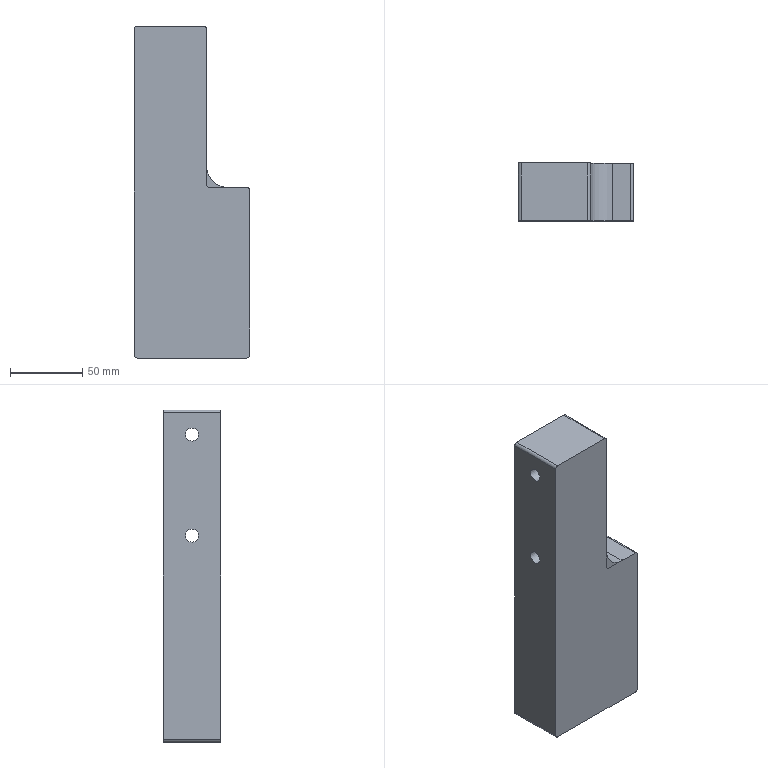NC program | NX | posted with a generic post | part box 80 x 40 x 230 mm
Lines 11596 to 12419 of 15398:
(PLANAR_MILL_COPY_COPY_1_COPY_1_COPY , TOOL : D10.)
N23148 T01 M6
N23150 G53
N23152 G17 G0 G90 X0.274 Y53.985 B0. C0. S3500 M3
N23154 G43 Z50. H1
N23156 Z4.6 B-180.
N23158 G41 G94 G1 X0.1 Y53. F1500. D1
N23160 Y38.
N23162 Y25.1
N23164 G3 X18.1 Y7.1 R18.
N23166 G1 X113.
N23168 X128.
N23170 G40
N23172 X128.985 Y7.274
N23174 G0 Z11.
N23176 X0.274 Y53.985
N23178 Z4.2
N23180 G41 G1 X0.1 Y53.
N23182 Y38.
N23184 Y25.1
N23186 G3 X18.1 Y7.1 R18.
N23188 G1 X113.
N23190 X128.
N23192 G40
N23194 X128.985 Y7.274
N23196 G0 Z10.6
N23198 X0.274 Y53.985
N23200 Z3.8
N23202 G41 G1 X0.1 Y53.
N23204 Y38.
N23206 Y25.1
N23208 G3 X18.1 Y7.1 R18.
N23210 G1 X113.
N23212 X128.
N23214 G40
N23216 X128.985 Y7.274
N23218 G0 Z10.2
N23220 X0.274 Y53.985
N23222 Z3.4
N23224 G41 G1 X0.1 Y53.
N23226 Y38.
N23228 Y25.1
N23230 G3 X18.1 Y7.1 R18.
N23232 G1 X113.
N23234 X128.
N23236 G40
N23238 X128.985 Y7.274
N23240 G0 Z9.8
N23242 X0.274 Y53.985
N23244 Z3.
N23246 G41 G1 X0.1 Y53.
N23248 Y38.
N23250 Y25.1
N23252 G3 X18.1 Y7.1 R18.
N23254 G1 X113.
N23256 X128.
N23258 G40
N23260 X128.985 Y7.274
N23262 G0 Z9.4
N23264 X0.274 Y53.985
N23266 Z2.6
N23268 G41 G1 X0.1 Y53.
N23270 Y38.
N23272 Y25.1
N23274 G3 X18.1 Y7.1 R18.
N23276 G1 X113.
N23278 X128.
N23280 G40
N23282 X128.985 Y7.274
N23284 G0 Z9.
N23286 X0.274 Y53.985
N23288 Z2.2
N23290 G41 G1 X0.1 Y53.
N23292 Y38.
N23294 Y25.1
N23296 G3 X18.1 Y7.1 R18.
N23298 G1 X113.
N23300 X128.
N23302 G40
N23304 X128.985 Y7.274
N23306 G0 Z8.6
N23308 X0.274 Y53.985
N23310 Z1.8
N23312 G41 G1 X0.1 Y53.
N23314 Y38.
N23316 Y25.1
N23318 G3 X18.1 Y7.1 R18.
N23320 G1 X113.
N23322 X128.
N23324 G40
N23326 X128.985 Y7.274
N23328 G0 Z8.2
N23330 X0.274 Y53.985
N23332 Z1.4
N23334 G41 G1 X0.1 Y53.
N23336 Y38.
N23338 Y25.1
N23340 G3 X18.1 Y7.1 R18.
N23342 G1 X113.
N23344 X128.
N23346 G40
N23348 X128.985 Y7.274
N23350 G0 Z7.8
N23352 X0.274 Y53.985
N23354 Z1.
N23356 G41 G1 X0.1 Y53.
N23358 Y38.
N23360 Y25.1
N23362 G3 X18.1 Y7.1 R18.
N23364 G1 X113.
N23366 X128.
N23368 G40
N23370 X128.985 Y7.274
N23372 G0 Z7.4
N23374 X0.274 Y53.985
N23376 Z0.6
N23378 G41 G1 X0.1 Y53.
N23380 Y38.
N23382 Y25.1
N23384 G3 X18.1 Y7.1 R18.
N23386 G1 X113.
N23388 X128.
N23390 G40
N23392 X128.985 Y7.274
N23394 G0 Z7.
N23396 X0.274 Y53.985
N23398 Z0.2
N23400 G41 G1 X0.1 Y53.
N23402 Y38.
N23404 Y25.1
N23406 G3 X18.1 Y7.1 R18.
N23408 G1 X113.
N23410 X128.
N23412 G40
N23414 X128.985 Y7.274
N23416 G0 Z6.6
N23418 X0.274 Y53.985
N23420 Z0.05
N23422 G41 G1 X0.1 Y53.
N23424 Y38.
N23426 Y25.1
N23428 G3 X18.1 Y7.1 R18.
N23430 G1 X113.
N23432 X128.
N23434 G40
N23436 X128.985 Y7.274
N23438 G0 Z50.
(ADAPTIVE_MILLING_COPY , TOOL : D10.)
N23440 X131.093 Y-42.154
N23442 Z3.05
N23444 G1 X130.949 Y-42.111 Z2.113 F3500.
N23446 X130.805 Y-42.068 Z1.742
N23448 X130.662 Y-42.025 Z1.47
N23450 X130.518 Y-41.982 Z1.25
N23452 X130.374 Y-41.939 Z1.066
N23454 X130.231 Y-41.896 Z0.908
N23456 X130.087 Y-41.853 Z0.77
N23458 X129.943 Y-41.81 Z0.65
N23460 X129.799 Y-41.767 Z0.545
N23462 X129.656 Y-41.724 Z0.452
N23464 X129.512 Y-41.681 Z0.371
N23466 X129.368 Y-41.638 Z0.3
N23468 X129.225 Y-41.595 Z0.24
N23470 X129.081 Y-41.552 Z0.188
N23472 X128.937 Y-41.509 Z0.145
N23474 X128.794 Y-41.466 Z0.111
N23476 X128.65 Y-41.423 Z0.084
N23478 X128.506 Y-41.38 Z0.065
N23480 X128.362 Y-41.337 Z0.054
N23482 X128.219 Y-41.294 Z0.05
N23484 X126.737 Y-40.85
N23486 G3 X125.467 Y-41.5 R1.047
N23488 G2 X123.725 Y-44.52 R40.399
N23490 X113.561 Y-50.458 R13.178
N23492 X107.135 Y-50.645 R78.774
N23494 G1 X-112.146 Y-50.635
N23496 G2 X-119.446 Y-48.637 R14.273
N23498 X-125.425 Y-38.867 R12.704
N23500 X-125.642 Y-32.835 R60.228
N23502 G1 X-125.639 Y36.996
N23504 G2 X-123.804 Y44.164 R14.479
N23506 X-113.788 Y50.434 R12.722
N23508 X-107.1 Y50.645 R72.946
N23510 G1 X0.181 Y50.637
N23512 G2 X7.374 Y48.74 R14.374
N23514 X13.522 Y38.896 R12.689
N23516 X13.745 Y32.297 R68.499
N23518 G3 X13.781 Y25.77 R248.361
N23520 X14.736 Y22.698 R5.595
N23522 X17.956 Y20.946 R4.399
N23524 X23.628 Y20.757 R59.107
N23526 G1 X111.896 Y20.742
N23528 G2 X118.927 Y19.038 R14.652
N23530 X125.426 Y8.959 R12.697
N23532 X125.642 Y2.928 R63.923
N23534 G1 X125.648 Y-36.497
N23536 G2 X123.98 Y-43.122 R12.586
N23538 X114.415 Y-49.838 R13.005
N23540 X108.618 Y-50.263 R39.297
N23542 X101.006 Y-50.3 R399.557
N23544 G1 X-111.196 Y-50.285
N23546 G2 X-117.348 Y-49.114 R16.471
N23548 X-124.778 Y-39.707 R12.409
N23550 X-125.256 Y-33.958 R35.302
N23552 X-125.299 Y-26.302 R339.034
N23554 G1 X-125.286 Y36.151
N23556 G2 X-124.163 Y42.228 R16.617
N23558 X-114.731 Y49.773 R12.402
N23560 X-108.721 Y50.261 R36.157
N23562 X-101.327 Y50.3 R362.187
N23564 G1 X-0.761 Y50.287
N23566 G2 X5.395 Y49.136 R16.577
N23568 X12.864 Y39.782 R12.391
N23570 X13.358 Y33.86 R35.329
N23572 G3 X13.435 Y26.558 R609.202
N23574 X14.161 Y23.314 R7.837
N23576 X17.726 Y20.79 R4.746
N23578 X22.393 Y20.443 R30.407
N23580 G1 X28.727 Y20.4
N23582 X111.114 Y20.387
N23584 G2 X117.231 Y19.262 R16.664
N23586 X124.759 Y9.903 R12.385
N23588 X125.257 Y4.025 R34.9
N23590 X125.3 Y-4.024 R361.131
N23592 G1 X125.289 Y-36.046
N23594 G2 X120.717 Y-46.35 R13.767
N23596 X114.248 Y-49.357 R13.562
N23598 X107.717 Y-49.904 R39.151
N23600 X100.017 Y-49.949 R337.307
N23602 G1 X-110.077 Y-49.939
N23604 G2 X-115.86 Y-49.124 R19.472
N23606 X-124.107 Y-40.288 R12.233
N23608 X-124.849 Y-34.484 R27.643
N23610 X-124.949 Y-24.816 R232.25
N23612 G1 X-124.936 Y35.259
N23614 G2 X-124.01 Y41.198 R18.667
N23616 X-115.359 Y49.088 R12.207
N23618 X-109.252 Y49.858 R28.129
N23620 X-99.803 Y49.949 R240.874
N23622 G1 X-1.753 Y49.938
N23624 G2 X4.068 Y49.089 R19.168
N23626 X12.203 Y40.301 R12.225
N23628 X12.954 Y34.366 R27.929
N23630 X13.08 Y27.438 R538.601
N23632 G3 X13.725 Y23.8 R10.769
N23634 X17.429 Y20.658 R5.131
N23636 X21.878 Y20.146 R22.319
N23638 X32.489 Y20.05 R321.794
N23640 G1 X110.277 Y20.036
N23642 G2 X116.173 Y19.119 R18.671
N23644 X124.094 Y10.433 R12.215
N23646 X124.845 Y4.674 R27.274
N23648 X124.949 Y-3.988 R198.27
N23650 G1 X124.938 Y-35.083
N23652 G2 X123.293 Y-42.177 R15.764
N23654 X115.323 Y-48.572 R12.671
N23656 X109.058 Y-49.472 R27.358
N23658 X98.122 Y-49.599 R259.091
N23660 G1 X-109.445 Y-49.585
N23662 G2 X-115.152 Y-48.832 R20.966
N23664 X-123.507 Y-40.447 R12.18
N23666 X-124.445 Y-34.498 R25.294
N23668 X-124.599 Y-23.825 R209.43
N23670 G1 X-124.588 Y34.27
N23672 G2 X-123.869 Y40.026 R21.602
N23674 X-115.528 Y48.482 R12.165
N23676 X-109.495 Y49.445 R25.079
N23678 X-100.397 Y49.598 R165.674
N23680 G1 X-2.642 Y49.588
N23682 G2 X3.03 Y48.897 R21.793
N23684 X11.599 Y40.475 R12.182
N23686 X12.556 Y34.309 R25.658
N23688 X12.739 Y27.832 R490.44
N23690 G3 X13.429 Y23.969 R12.316
N23692 X17.415 Y20.456 R5.669
N23694 X22.181 Y19.827 R22.029
N23696 X31.484 Y19.7 R199.522
N23698 G1 X109.321 Y19.688
N23700 G2 X115.117 Y18.942 R21.289
N23702 X123.491 Y10.599 R12.168
N23704 X124.45 Y4.521 R25.332
N23706 X124.598 Y-4.796 R186.673
N23708 G1 X124.586 Y-34.202
N23710 G2 X123.484 Y-40.504 R17.988
N23712 X115.532 Y-47.956 R12.572
N23714 X109.214 Y-49.061 R24.942
N23716 X100.293 Y-49.247 R142.121
N23718 G1 X-108.576 Y-49.236
N23720 G2 X-114.425 Y-48.542 R23.063
N23722 X-122.924 Y-40.51 R12.175
N23724 X-124.044 Y-34.373 R23.938
N23726 X-124.247 Y-25.321 R141.619
N23728 G1 X-124.235 Y33.616
N23730 G2 X-123.555 Y39.379 R23.087
N23732 X-115.513 Y47.923 R12.178
N23734 X-109.377 Y49.044 R23.937
N23736 X-99.45 Y49.248 R154.683
N23738 G1 X-3.281 Y49.235
N23740 G2 X2.524 Y48.542 R22.961
N23742 X11.021 Y40.522 R12.172
N23744 X12.156 Y34.211 R24.261
N23746 X12.401 Y28.105 R502.905
N23748 G3 X13.157 Y24.057 R13.32
N23750 X17.299 Y20.275 R6.168
N23752 X22.116 Y19.527 R20.663
N23754 X31.879 Y19.35 R179.371
N23756 G1 X108.664 Y19.335
N23758 G2 X114.51 Y18.618 R22.679
N23760 X122.918 Y10.626 R12.171
N23762 X124.046 Y4.445 R23.951
N23764 X124.246 Y-4.432 R136.352
N23766 G1 X124.234 Y-33.42
N23768 G2 X123.335 Y-39.454 R20.013
N23770 X115.476 Y-47.417 R12.566
N23772 X109.009 Y-48.667 R24.183
N23774 X100.045 Y-48.895 R130.758
N23776 G1 X-107.827 Y-48.886
N23778 G2 X-113.685 Y-48.252 R25.051
N23780 X-122.425 Y-40.317 R12.256
N23782 X-123.659 Y-34.024 R23.668
N23784 X-123.893 Y-25.411 R121.991
N23786 G1 X-123.885 Y32.827
N23788 G2 X-123.284 Y38.557 R25.399
N23790 X-115.388 Y47.398 R12.244
N23792 X-109.056 Y48.656 R23.442
N23794 X-99.962 Y48.895 R126.676
N23796 G1 X-4.042 Y48.885
N23798 G2 X1.815 Y48.244 R24.896
N23800 X10.499 Y40.388 R12.237
N23802 X11.749 Y34.143 R23.32
N23804 X12.06 Y28.335 R420.196
N23806 G3 X12.949 Y23.966 R14.108
N23808 X17.196 Y20.085 R6.681
N23810 X21.97 Y19.237 R19.678
N23812 X31.014 Y19.005 R133.329
N23814 G1 X107.914 Y18.985
N23816 G2 X113.685 Y18.352 R24.815
N23818 X122.388 Y10.516 R12.231
N23820 X123.643 Y4.317 R23.118
N23822 X123.894 Y-4.778 R120.904
N23824 G1 X123.889 Y-32.259
N23826 G2 X123.234 Y-38.113 R23.956
N23828 X115.235 Y-46.945 R12.637
N23830 X108.914 Y-48.262 R23.609
N23832 X100.127 Y-48.541 R110.359
N23834 G1 X-107.035 Y-48.536
N23836 G2 X-112.86 Y-47.977 R27.616
N23838 X-121.933 Y-40.111 R12.352
N23840 X-123.271 Y-33.707 R23.354
N23842 X-123.542 Y-24.657 R115.958
N23844 G1 X-123.533 Y32.224
N23846 G2 X-122.913 Y38.129 R26.218
N23848 X-115.244 Y46.88 R12.306
N23850 X-108.978 Y48.246 R22.651
N23852 X-100.104 Y48.541 R105.687
N23854 G1 X-4.679 Y48.533
N23856 G2 X1.14 Y47.934 R26.427
N23858 X10.024 Y40.132 R12.333
N23860 X11.37 Y33.729 R23.327
N23862 G3 X11.759 Y28.099 R694.113
N23864 X12.8 Y23.736 R13.63
N23866 X17.17 Y19.863 R7.234
N23868 X22.057 Y18.932 R19.665
N23870 X31.672 Y18.655 R125.783
N23872 G1 X107.219 Y18.634
N23874 G2 X112.996 Y18.045 R26.596
N23876 X121.936 Y10.202 R12.346
N23878 X123.276 Y3.754 R23.451
N23880 X123.542 Y-5.077 R114.881
N23882 G1 X123.536 Y-31.67
N23884 G2 X122.893 Y-37.571 R25.133
N23886 X115.093 Y-46.434 R12.673
N23888 X108.492 Y-47.887 R23.413
N23890 X99.137 Y-48.191 R111.429
N23892 G1 X-106.47 Y-48.184
N23894 G2 X-112.382 Y-47.618 R28.359
N23896 X-121.489 Y-39.788 R12.455
N23898 X-122.884 Y-33.396 R23.229
N23900 X-123.188 Y-24.698 R103.453
N23902 G1 X-123.187 Y31.252
N23904 G2 X-122.675 Y37.126 R30.064
N23906 X-118.101 Y44.631 R12.469
N23908 X-111.849 Y47.368 R15.515
N23910 X-104.896 Y48.099 R39.966
N23912 X-93.872 Y48.198 R302.972
N23914 G1 X-5.442 Y48.184
N23916 G2 X0.513 Y47.612 R28.32
N23918 X9.559 Y39.861 R12.438
N23920 X10.981 Y33.474 R23.211
N23922 G3 X11.449 Y28.016 R259.571
N23924 X12.625 Y23.571 R13.849
N23926 X17.138 Y19.637 R7.798
N23928 X22.297 Y18.612 R20.186
N23930 X31.853 Y18.308 R118.944
N23932 G1 X106.471 Y18.285
N23934 G2 X112.34 Y17.729 R28.522
N23936 X121.449 Y9.986 R12.437
N23938 X122.874 Y3.602 R22.893
N23940 X123.187 Y-5.096 R100.525
N23942 G1 X123.186 Y-30.915
N23944 G2 X122.612 Y-36.781 R27.524
N23946 X114.658 Y-46.044 R12.797
N23948 X108.235 Y-47.496 R23.405
N23950 X99.451 Y-47.834 R97.738
N23952 G1 X-105.611 Y-47.837
N23954 G2 X-111.532 Y-47.342 R31.559
N23956 X-118.935 Y-43.055 R12.628
N23958 X-121.91 Y-36.725 R15.278
N23960 X-122.722 Y-29.827 R37.431
N23962 X-122.848 Y-18.365 R308.19
N23964 G1 X-122.837 Y30.553
N23966 G2 X-122.345 Y36.518 R31.863
N23968 X-118.14 Y43.863 R12.641
N23970 X-111.964 Y46.852 R14.99
N23972 X-104.897 Y47.719 R36.261
N23974 X-93.392 Y47.848 R302.118
N23976 G1 X-6.324 Y47.837
N23978 G2 X-0.317 Y47.332 R31.493
N23980 X7.206 Y42.843 R12.587
N23982 X10.044 Y36.582 R15.539
N23984 X10.864 Y30.428 R45.557
N23986 G3 X11.667 Y25.393 R26.942
N23988 X14.38 Y20.967 R8.85
N23990 X18.692 Y18.909 R10.574
N23992 X24.902 Y18.12 R32.956
N23994 X35.772 Y17.949 R241.455
N23996 G1 X105.557 Y17.938
N23998 G2 X111.478 Y17.454 R32.015
N24000 X118.752 Y13.372 R12.681
N24002 X121.862 Y7.023 R15.005
N24004 X122.713 Y0.13 R36.108
N24006 X122.848 Y-11.418 R290.381
N24008 G1 X122.834 Y-30.358
N24010 G2 X122.263 Y-36.269 R28.459
N24012 X114.507 Y-45.541 R12.848
N24014 X107.89 Y-47.115 R23.083
N24016 X98.845 Y-47.483 R95.445
N24018 G1 X-104.983 Y-47.486
N24020 G2 X-110.992 Y-46.998 R32.777
N24022 X-118.475 Y-42.714 R12.751
N24024 X-121.52 Y-36.311 R15.438
N24026 X-122.37 Y-29.153 R38.015
N24028 X-122.497 Y-17.299 R320.42
N24030 G1 X-122.483 Y30.202
N24032 G2 X-121.972 Y36.12 R31.4
N24034 X-117.219 Y43.867 R12.659
N24036 X-110.841 Y46.627 R16.105
N24038 X-103.629 Y47.39 R41.585
N24040 X-92.298 Y47.497 R363.499
N24042 G1 X-6.886 Y47.486
N24044 G2 X-0.835 Y46.984 R32.349
N24046 X6.764 Y42.482 R12.708
N24048 X9.657 Y36.163 R15.742
N24050 X10.507 Y30.376 R47.607
N24052 G3 X11.417 Y25.294 R27.085
N24054 X14.586 Y20.533 R9.219
N24056 X19.239 Y18.511 R12.12
N24058 X25.918 Y17.749 R38.379
N24060 X37.564 Y17.598 R299.62
N24062 G1 X104.983 Y17.587
N24064 G2 X111.035 Y17.09 R32.587
N24066 X118.495 Y12.79 R12.732
N24068 X121.525 Y6.393 R15.451
N24070 X122.374 Y-0.853 R38.45
N24072 X122.497 Y-12.576 R326.291
N24074 G1 X122.485 Y-29.601
N24076 G2 X121.94 Y-35.647 R30.419
N24078 X114.121 Y-45.138 R12.958
N24080 X107.642 Y-46.724 R22.982
N24082 X98.818 Y-47.127 R87.849
N24084 G1 X91.643 Y-47.147
N24086 X-104.32 Y-47.136
N24088 G2 X-110.332 Y-46.678 R34.785
N24090 X-117.453 Y-42.998 R13.039
N24092 X-120.956 Y-36.582 R14.748
N24094 X-121.97 Y-29.491 R33.516
N24096 X-122.146 Y-19.125 R199.152
N24098 G1 X-122.136 Y29.312
N24100 G2 X-121.672 Y35.368 R34.557
N24102 X-117.804 Y42.637 R12.989
N24104 X-111.539 Y45.967 R14.883
N24106 X-104.492 Y46.97 R33.647
N24108 X-92.507 Y47.147 R242.977
N24110 G1 X-7.582 Y47.136
N24112 G2 X-1.527 Y46.671 R34.497
N24114 X5.739 Y42.802 R12.984
N24116 X9.068 Y36.551 R14.942
N24118 X10.02 Y31.346 R34.859
N24120 G3 X10.918 Y26.022 R39.676
N24122 X13.473 Y21.232 R10.716
N24124 X18.179 Y18.526 R10.794
N24126 X24.311 Y17.524 R28.636
N24128 X33.996 Y17.258 R149.398
N24130 G1 X104.333 Y17.237
N24132 G2 X110.431 Y16.76 R34.28
N24134 X117.763 Y12.767 R12.941
N24136 X121.022 Y6.436 R15.089
N24138 X121.977 Y-0.531 R34.606
N24140 X122.147 Y-11.51 R230.562
N24142 G1 X122.133 Y-29.045
N24144 G2 X121.629 Y-34.965 R32.049
N24146 X117.032 Y-42.77 R13.102
N24148 X110.613 Y-45.765 R16.137
N24150 X103.153 Y-46.661 R39.462
N24152 X90.555 Y-46.797 R331.416
N24154 G1 X-103.845 Y-46.784
N24156 G2 X-109.815 Y-46.331 R35.248
N24158 X-116.993 Y-42.66 R13.179
N24160 X-120.56 Y-36.203 R14.847
N24162 X-121.604 Y-29.119 R33.287
N24164 X-121.796 Y-17.965 R212.844
N24166 G1 X-121.782 Y29.02
N24168 G2 X-121.272 Y35.115 R32.987
N24170 X-116.589 Y42.928 R12.904
N24172 X-110.297 Y45.795 R16.136
N24174 X-102.878 Y46.666 R39.803
N24176 X-90.585 Y46.797 R333.437
N24178 G1 X-7.848 Y46.781
N24180 G2 X-1.797 Y46.275 R32.957
N24182 X7.865 Y38.461 R12.928
N24184 X9.442 Y32.601 R24.348
N24186 G3 X10.329 Y27.196 R97.299
N24188 X12.251 Y22.381 R13.7
N24190 X17.324 Y18.552 R10.31
N24192 X23.342 Y17.298 R24.031
N24194 X33.18 Y16.917 R113.098
N24196 G1 X41.543 Y16.898
N24198 X104.02 Y16.883
N24200 G2 X110.115 Y16.373 R33.025
N24202 X117.866 Y11.769 R12.914
N24204 X120.813 Y5.319 R16.137
N24206 X121.66 Y-1.884 R39.651
N24208 X121.797 Y-14.263 R321.24
N24210 G1 X121.78 Y-28.62
N24212 G2 X121.238 Y-34.667 R31.508
N24214 X113.331 Y-44.349 R13.167
N24216 X106.686 Y-45.998 R23.448
N24218 X97.687 Y-46.423 R88.148
N24220 G1 X90.031 Y-46.447
N24222 X-103.088 Y-46.436
N24224 G2 X-109.19 Y-46.003 R37.533
N24226 X-116.169 Y-42.677 R13.46
N24228 X-120.016 Y-36.324 R14.481
N24230 X-121.199 Y-29.352 R30.367
N24232 X-121.443 Y-19.076 R156.13
N24234 G1 X-121.436 Y28.093
N24236 G2 X-120.987 Y34.281 R36.989
N24238 X-117.515 Y41.34 R13.363
N24240 X-111.06 Y45.098 R14.709
N24242 X-103.945 Y46.226 R32.001
N24244 X-92.355 Y46.446 R199.332
N24246 G1 X-8.83 Y46.436
N24248 G2 X-2.641 Y45.991 R37.258
N24250 X4.452 Y42.503 R13.38
N24252 X8.145 Y36.271 R14.772
N24254 X9.251 Y31.323 R33.759
N24256 G3 X10.332 Y25.99 R44.29
N24258 X13.17 Y20.901 R11.86
N24260 X18.276 Y17.959 R12.01
N24262 X24.689 Y16.867 R29.997
N24264 X34.876 Y16.56 R145.374
N24266 G1 X103.105 Y16.537
N24268 G2 X109.207 Y16.101 R37.359
N24270 X116.253 Y12.698 R13.433
N24272 X120.07 Y6.249 R14.616
N24274 X121.223 Y-0.905 R31.645
N24276 X121.444 Y-11.007 R164.918
N24278 G1 X121.432 Y-27.864
N24280 G2 X120.924 Y-34.003 R33.789
N24282 X116.592 Y-41.688 R13.348
N24284 X110.13 Y-44.922 R15.947
N24286 X102.729 Y-45.921 R37.025
N24288 X92.056 Y-46.095 R206.92
N24290 G1 X-102.839 Y-46.082
N24292 G2 X-109.024 Y-45.592 R35.136
N24294 X-116.499 Y-41.545 R13.274
N24296 X-119.87 Y-35.113 R15.495
N24298 X-120.895 Y-28.025 R34.756
N24300 X-121.095 Y-17.003 R207.337
N24302 G1 X-121.081 Y27.839
N24304 G2 X-120.608 Y33.938 R35.587
N24306 X-116.781 Y41.279 R13.348
N24308 X-110.36 Y44.8 R15.206
N24310 X-103.236 Y45.882 R33.514
N24312 X-91.995 Y46.095 R200.244
N24314 G1 X-9.073 Y46.082
N24316 G2 X-2.888 Y45.594 R35.239
N24318 X4.595 Y41.551 R13.281
N24320 X7.893 Y35.48 R15.667
N24322 X9.168 Y29.659 R52.676
N24324 G3 X10.593 Y24.428 R25.72
N24326 X17.244 Y18.046 R11.311
N24328 X23.635 Y16.653 R25.135
N24330 X33.281 Y16.227 R105.798
N24332 G1 X44.475 Y16.198
N24334 X102.883 Y16.182
N24336 G2 X109.024 Y15.692 R34.901
N24338 X116.525 Y11.617 R13.269
N24340 X119.901 Y5.096 R15.588
N24342 X120.914 Y-2.215 R35.979
N24344 X121.095 Y-12.931 R203.177
N24346 G1 X121.079 Y-27.418
N24348 G2 X120.565 Y-33.557 R33.938
N24350 X116.21 Y-41.286 R13.444
N24352 X109.749 Y-44.537 R16.055
N24354 X102.438 Y-45.554 R36.605
N24356 X90.672 Y-45.746 R234.087
N24358 G1 X-101.877 Y-45.736
N24360 G2 X-108.069 Y-45.326 R40.381
N24362 X-114.981 Y-42.245 R13.906
N24364 X-119.181 Y-35.725 R14.462
N24366 X-120.456 Y-28.726 R29.583
N24368 X-120.741 Y-18.32 R145.964
N24370 G1 X-120.736 Y26.877
N24372 G2 X-120.325 Y33.069 R40.367
N24374 X-117.213 Y40.017 R13.891
N24376 X-110.8 Y44.155 R14.443
N24378 X-103.762 Y45.453 R29.337
N24380 X-93.312 Y45.741 R145.575
N24382 G1 X-9.918 Y45.735
N24384 G2 X-3.77 Y45.315 R39.508
N24386 X3.222 Y42.122 R13.83
N24388 X7.207 Y36.024 R14.711
N24390 X8.515 Y31.078 R33.756
N24392 G3 X9.843 Y25.621 R44.721
N24394 X13.202 Y20.224 R12.664
N24396 X18.772 Y17.257 R13.735
N24398 X25.872 Y16.142 R34.748
N24400 X36.794 Y15.856 R173.894
N24402 G1 X102.02 Y15.835
N24404 G2 X108.296 Y15.387 R38.29
N24406 X115.411 Y11.957 R13.656
N24408 X119.292 Y5.481 R14.831
N24410 X120.499 Y-1.753 R31.622
N24412 X120.744 Y-12.73 R175.896
N24414 X120.708 Y-27.864 R882.062
N24416 X120.009 Y-33.98 R27.735
N24418 X112.28 Y-43.126 R13.393
N24420 X105.398 Y-44.902 R23.651
N24422 X96.621 Y-45.362 R83.736
N24424 G1 X87.959 Y-45.396
N24426 X-101.485 Y-45.384
N24428 G2 X-107.633 Y-44.966 R40.002
N24430 X-114.587 Y-41.854 R13.99
N24432 X-118.81 Y-35.291 R14.585
N24434 X-120.098 Y-28.249 R29.851
N24436 X-120.39 Y-17.668 R147.013
N24438 G1 X-120.384 Y26.482
N24440 G2 X-119.944 Y32.759 R39.242
N24442 X-116.722 Y39.738 R13.878
N24444 X-110.199 Y43.84 R14.705
N24446 X-103.11 Y45.109 R30.352
N24448 X-92.747 Y45.39 R145.068
N24450 G1 X-10.648 Y45.386
N24452 G2 X-4.281 Y44.968 R41.261
N24454 X2.641 Y41.896 R14.034
N24456 X6.785 Y35.772 R14.793
N24458 X8.211 Y30.677 R35.375
N24460 G3 X9.671 Y25.247 R40.407
N24462 X13.729 Y19.464 R12.824
N24464 X19.459 Y16.786 R15.395
N24466 X26.874 Y15.753 R40.013
N24468 X39.19 Y15.499 R222.897
N24470 G1 X101.487 Y15.485
N24472 G2 X107.808 Y15.036 R38.976
N24474 X114.946 Y11.633 R13.798
N24476 X118.904 Y5.1 R14.902
N24478 X120.134 Y-2.13 R31.538
N24480 X120.392 Y-12.975 R167.463
N24482 X120.355 Y-27.426 R839.812
N24484 X119.651 Y-33.542 R27.828
N24486 X111.8 Y-42.782 R13.507
N24488 X104.916 Y-44.545 R23.989
N24490 X95.92 Y-45.013 R85.415
N24492 G1 X87.651 Y-45.046
N24494 X-101.18 Y-45.03
N24496 G2 X-107.369 Y-44.577 R38.242
N24498 X-114.575 Y-41.124 R13.891
N24500 X-118.496 Y-34.689 R14.98
N24502 X-119.768 Y-27.422 R31.212
N24504 X-120.041 Y-16.797 R156.215
N24506 G1 X-120.032 Y26.046
N24508 G2 X-119.585 Y32.323 R39.154
N24510 X-116.24 Y39.449 R13.944
N24512 X-109.709 Y43.49 R14.911
N24514 X-102.4 Y44.77 R31.257
N24516 X-91.555 Y45.042 R162.418
N24518 G1 X-11.005 Y45.034
N24520 G2 X-4.769 Y44.618 R41.024
N24522 X2.201 Y41.549 R14.179
N24524 X6.368 Y35.515 R14.963
N24526 X7.856 Y30.53 R35.164
N24528 G3 X9.452 Y25.015 R40.957
N24530 X14.059 Y18.914 R13.237
N24532 X20.091 Y16.342 R16.943
N24534 X28.134 Y15.355 R46.215
N24536 X40.107 Y15.148 R244.365
N24538 G1 X100.873 Y15.135
N24540 G2 X107.196 Y14.708 R40.72
N24542 X114.184 Y11.575 R14.091
N24544 X118.39 Y5.109 R14.646
N24546 X119.724 Y-1.923 R29.353
N24548 X120.037 Y-11.934 R130.889
N24550 X120.002 Y-26.99 R783.022
N24552 X119.292 Y-33.105 R27.948
N24554 X111.523 Y-42.348 R13.572
N24556 X104.784 Y-44.145 R23.551
N24558 X95.704 Y-44.657 R80.55
N24560 G1 X87.129 Y-44.695
N24562 X-100.434 Y-44.683
N24564 G2 X-106.713 Y-44.257 R40.981
N24566 X-113.652 Y-41.208 R14.266
N24568 X-118.021 Y-34.58 R14.704
N24570 X-119.382 Y-27.329 R29.96
N24572 X-119.688 Y-16.88 R141.175
N24574 G1 X-119.68 Y25.607
N24576 G2 X-119.228 Y31.884 R39.112
N24578 X-115.901 Y39.005 R14.058
N24580 X-109.43 Y43.072 R14.928
N24582 X-102.216 Y44.391 R30.521
N24584 X-92.029 Y44.688 R140.674
N24586 G1 X-11.436 Y44.682
N24588 G2 X-5.028 Y44.23 R39.929
N24590 X2.207 Y40.814 R14.077
N24592 X6.149 Y34.778 R15.722
N24594 X7.842 Y29.086 R53.078
N24596 G3 X9.754 Y23.656 R27.865
N24598 X17.268 Y16.922 R13.599
N24600 X24.044 Y15.368 R27.456
N24602 X34. Y14.844 R99.657
N24604 X48.41 Y14.797 R846.501
N24606 G1 X100.433 Y14.784
N24608 G2 X106.712 Y14.358 R40.968
N24610 X113.759 Y11.218 R14.236
N24612 X118.024 Y4.674 R14.756
N24614 X119.364 Y-2.357 R29.558
N24616 X119.685 Y-12.28 R126.711
N24618 X119.651 Y-26.508 R698.507
N24620 X118.936 Y-32.666 R28.195
N24622 X111.116 Y-41.974 R13.661
N24624 X104.249 Y-43.797 R23.829
N24626 X95.212 Y-44.306 R81.594
N24628 X85.981 Y-44.345 R596.713
N24630 G1 X-99.952 Y-44.332
N24632 G2 X-106.404 Y-43.878 R40.458
N24634 X-113.509 Y-40.61 R14.213
N24636 X-117.716 Y-33.971 R15.012
N24638 X-119.027 Y-26.844 R30.47
N24640 X-119.337 Y-16.482 R141.062
N24642 G1 X-119.335 Y24.602
N24644 G2 X-118.936 Y31.059 R44.421
N24646 X-116.114 Y37.904 R14.633
N24648 X-109.549 Y42.514 R14.518
N24650 X-102.583 Y43.961 R28.055
N24652 X-92.574 Y44.331 R117.347
N24654 G1 X-12.374 Y44.336
N24656 G2 X-5.917 Y43.948 R45.481
N24658 X0.958 Y41.154 R14.739
N24660 X5.496 Y35.119 R15.071
N24662 X7.164 Y30.182 R35.465
N24664 G3 X8.962 Y24.686 R42.982
N24666 X14.514 Y18.009 R14.27
N24668 X20.976 Y15.557 R19.616
N24670 X29.585 Y14.626 R54.287
N24672 X43.339 Y14.445 R355.381
N24674 G1 X99.824 Y14.434
N24676 G2 X106.234 Y14.008 R42.027
N24678 X113.254 Y10.93 R14.391
N24680 X117.605 Y4.395 R14.756
N24682 X118.994 Y-2.671 R29.185
N24684 X119.335 Y-13.075 R130.456
N24686 X119.292 Y-26.25 R543.955
N24688 X118.546 Y-32.36 R27.458
N24690 X110.703 Y-41.606 R13.746
N24692 X103.66 Y-43.457 R24.221
N24694 X94.579 Y-43.956 R83.971
N24696 X85.96 Y-43.995 R587.256
N24698 G1 X-99.546 Y-43.98
N24700 G2 X-105.911 Y-43.531 R40.524
N24702 X-113.036 Y-40.3 R14.375
N24704 X-117.299 Y-33.698 R15.019
N24706 X-118.662 Y-26.494 R30.306
N24708 X-118.987 Y-15.827 R140.665
N24710 G1 X-118.98 Y24.517
N24712 G2 X-118.521 Y30.969 R40.306
N24714 X-115.313 Y38.021 R14.332
N24716 X-108.773 Y42.273 R14.968
N24718 X-101.66 Y43.647 R29.805
N24720 X-91.343 Y43.985 R132.148
N24722 G1 X-12.368 Y43.98
N24724 G2 X-6.003 Y43.534 R40.749
N24726 X1.273 Y40.194 R14.437
N24728 X5.349 Y34.268 R16.104
N24730 X7.124 Y28.998 R51.89
N24732 G3 X9.292 Y23.341 R30.84
N24734 X17.256 Y16.352 R14.763
N24736 X24.44 Y14.697 R29.123
N24738 X34.746 Y14.147 R102.641
N24740 X48.462 Y14.096 R786.315
N24742 G1 X99.602 Y14.08
N24744 G2 X105.966 Y13.622 R39.903
N24746 X113.077 Y10.364 R14.328
N24748 X117.302 Y3.788 R15.035
N24750 X118.666 Y-3.463 R30.45
N24752 X118.987 Y-14.086 R141.887
N24754 X118.927 Y-26.161 R393.285
N24756 X118.086 Y-32.3 R25.706
N24758 X110.345 Y-41.213 R13.803
N24760 X103.438 Y-43.071 R24.021
N24762 X94.49 Y-43.598 R79.701
N24764 X85.478 Y-43.645 R517.917
N24766 G1 X-98.814 Y-43.632
N24768 G2 X-105.356 Y-43.196 R42.781
N24770 X-112.377 Y-40.148 R14.621
N24772 X-116.826 Y-33.584 R14.869
N24774 X-118.265 Y-26.484 R29.033
N24776 X-118.632 Y-16.081 R124.816
N24778 G1 X-118.636 Y23.431
N24780 G2 X-118.249 Y30.02 R47.238
N24782 X-115.572 Y36.835 R15.046